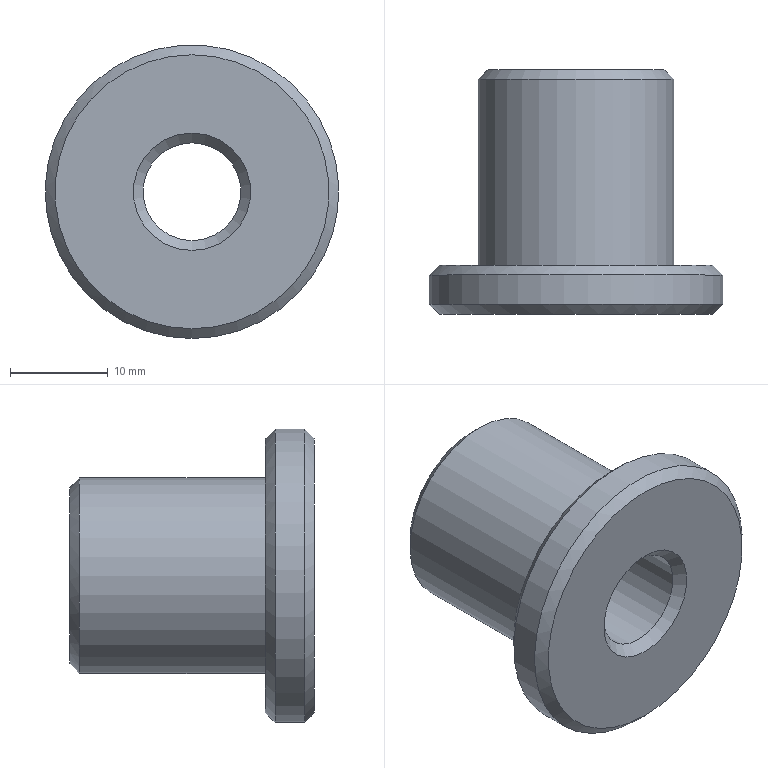Part | NX | features solid 2 | 1 solid | 10 faces | box 30 x 25 x 30 mm | volume 7715 mm3 | cone 4 | plane 3 | cylinder 3 | commonest cylinder face diameters 10 x1 20 x1 30 x1
STEP:
#1=CARTESIAN_POINT('',(0.000006093,336.216,159.366));
#2=VERTEX_POINT('',#1);
#3=CARTESIAN_POINT('',(0.000006093,336.216,173.366));
#4=DIRECTION('',(0.,-1.,0.));
#5=DIRECTION('',(0.,0.,-1.));
#6=AXIS2_PLACEMENT_3D('',#3,#4,#5);
#7=CIRCLE('',#6,14.);
#8=EDGE_CURVE('',#2,#2,#7,.F.);
#9=ORIENTED_EDGE('',*,*,#8,.T.);
#10=EDGE_LOOP('',(#9));
#11=FACE_BOUND('',#10,.T.);
#12=CARTESIAN_POINT('',(0.000006093,336.216,163.366));
#13=VERTEX_POINT('',#12);
#14=CARTESIAN_POINT('',(0.000006093,336.216,173.366));
#15=DIRECTION('',(0.,-1.,0.));
#16=DIRECTION('',(0.,0.,-1.));
#17=AXIS2_PLACEMENT_3D('',#14,#15,#16);
#18=CIRCLE('',#17,10.);
#19=EDGE_CURVE('',#13,#13,#18,.T.);
#20=ORIENTED_EDGE('',*,*,#19,.T.);
#21=EDGE_LOOP('',(#20));
#22=FACE_BOUND('',#21,.T.);
#23=CARTESIAN_POINT('',(-0.000000942,336.216,122.381));
#24=DIRECTION('',(0.,-1.,0.));
#25=DIRECTION('',(-1.,0.,0.));
#26=AXIS2_PLACEMENT_3D('',#23,#24,#25);
#27=PLANE('',#26);
#28=ADVANCED_FACE('',(#11,#22),#27,.F.);
#29=CARTESIAN_POINT('',(0.000006093,331.216,167.366));
#30=VERTEX_POINT('',#29);
#31=CARTESIAN_POINT('',(0.000006093,331.216,173.366));
#32=DIRECTION('',(0.,-1.,0.));
#33=DIRECTION('',(0.,0.,-1.));
#34=AXIS2_PLACEMENT_3D('',#31,#32,#33);
#35=CIRCLE('',#34,6.);
#36=EDGE_CURVE('',#30,#30,#35,.F.);
#37=ORIENTED_EDGE('',*,*,#36,.T.);
#38=EDGE_LOOP('',(#37));
#39=FACE_BOUND('',#38,.T.);
#40=CARTESIAN_POINT('',(0.000006093,331.216,159.366));
#41=VERTEX_POINT('',#40);
#42=CARTESIAN_POINT('',(0.000006093,331.216,173.366));
#43=DIRECTION('',(0.,-1.,0.));
#44=DIRECTION('',(0.,0.,-1.));
#45=AXIS2_PLACEMENT_3D('',#42,#43,#44);
#46=CIRCLE('',#45,14.);
#47=EDGE_CURVE('',#41,#41,#46,.T.);
#48=ORIENTED_EDGE('',*,*,#47,.T.);
#49=EDGE_LOOP('',(#48));
#50=FACE_BOUND('',#49,.T.);
#51=CARTESIAN_POINT('',(-0.000000942,331.216,122.381));
#52=DIRECTION('',(0.,-1.,0.));
#53=DIRECTION('',(-1.,0.,0.));
#54=AXIS2_PLACEMENT_3D('',#51,#52,#53);
#55=PLANE('',#54);
#56=ADVANCED_FACE('',(#39,#50),#55,.T.);
#57=CARTESIAN_POINT('',(0.000006093,335.216,158.366));
#58=VERTEX_POINT('',#57);
#59=CARTESIAN_POINT('',(0.000006093,335.216,173.366));
#60=DIRECTION('',(0.,-1.,0.));
#61=DIRECTION('',(0.,0.,-1.));
#62=AXIS2_PLACEMENT_3D('',#59,#60,#61);
#63=CIRCLE('',#62,15.);
#64=EDGE_CURVE('',#58,#58,#63,.T.);
#65=ORIENTED_EDGE('',*,*,#64,.T.);
#66=EDGE_LOOP('',(#65));
#67=FACE_BOUND('',#66,.T.);
#68=CARTESIAN_POINT('',(0.000006093,332.216,158.366));
#69=VERTEX_POINT('',#68);
#70=CARTESIAN_POINT('',(0.000006093,332.216,173.366));
#71=DIRECTION('',(0.,-1.,0.));
#72=DIRECTION('',(0.,0.,-1.));
#73=AXIS2_PLACEMENT_3D('',#70,#71,#72);
#74=CIRCLE('',#73,15.);
#75=EDGE_CURVE('',#69,#69,#74,.F.);
#76=ORIENTED_EDGE('',*,*,#75,.T.);
#77=EDGE_LOOP('',(#76));
#78=FACE_BOUND('',#77,.T.);
#79=CARTESIAN_POINT('',(0.000006093,361.216,173.366));
#80=DIRECTION('',(0.,-1.,0.));
#81=DIRECTION('',(1.,0.,0.));
#82=AXIS2_PLACEMENT_3D('',#79,#80,#81);
#83=CYLINDRICAL_SURFACE('',#82,15.);
#84=ADVANCED_FACE('',(#67,#78),#83,.T.);
#85=CARTESIAN_POINT('',(0.000006093,356.216,182.366));
#86=VERTEX_POINT('',#85);
#87=CARTESIAN_POINT('',(0.000006093,356.216,173.366));
#88=DIRECTION('',(0.,1.,0.));
#89=DIRECTION('',(0.,0.,1.));
#90=AXIS2_PLACEMENT_3D('',#87,#88,#89);
#91=CIRCLE('',#90,9.);
#92=EDGE_CURVE('',#86,#86,#91,.T.);
#93=ORIENTED_EDGE('',*,*,#92,.T.);
#94=EDGE_LOOP('',(#93));
#95=FACE_BOUND('',#94,.T.);
#96=CARTESIAN_POINT('',(0.000006093,356.216,178.366));
#97=VERTEX_POINT('',#96);
#98=CARTESIAN_POINT('',(0.000006093,356.216,173.366));
#99=DIRECTION('',(0.,1.,0.));
#100=DIRECTION('',(0.,0.,1.));
#101=AXIS2_PLACEMENT_3D('',#98,#99,#100);
#102=CIRCLE('',#101,5.);
#103=EDGE_CURVE('',#97,#97,#102,.T.);
#104=ORIENTED_EDGE('',*,*,#103,.F.);
#105=EDGE_LOOP('',(#104));
#106=FACE_BOUND('',#105,.T.);
#107=CARTESIAN_POINT('',(0.000006093,356.216,173.366));
#108=DIRECTION('',(0.,1.,0.));
#109=DIRECTION('',(0.,0.,1.));
#110=AXIS2_PLACEMENT_3D('',#107,#108,#109);
#111=PLANE('',#110);
#112=ADVANCED_FACE('',(#95,#106),#111,.T.);
#113=CARTESIAN_POINT('',(0.000006093,355.216,183.366));
#114=VERTEX_POINT('',#113);
#115=CARTESIAN_POINT('',(0.000006093,355.216,173.366));
#116=DIRECTION('',(0.,1.,0.));
#117=DIRECTION('',(0.,0.,1.));
#118=AXIS2_PLACEMENT_3D('',#115,#116,#117);
#119=CIRCLE('',#118,10.);
#120=EDGE_CURVE('',#114,#114,#119,.F.);
#121=ORIENTED_EDGE('',*,*,#120,.T.);
#122=EDGE_LOOP('',(#121));
#123=FACE_BOUND('',#122,.T.);
#124=ORIENTED_EDGE('',*,*,#19,.F.);
#125=EDGE_LOOP('',(#124));
#126=FACE_BOUND('',#125,.T.);
#127=CARTESIAN_POINT('',(0.000006093,361.216,173.366));
#128=DIRECTION('',(0.,-1.,0.));
#129=DIRECTION('',(1.,0.,0.));
#130=AXIS2_PLACEMENT_3D('',#127,#128,#129);
#131=CYLINDRICAL_SURFACE('',#130,10.);
#132=ADVANCED_FACE('',(#123,#126),#131,.T.);
#133=CARTESIAN_POINT('',(0.000006093,332.216,168.366));
#134=VERTEX_POINT('',#133);
#135=CARTESIAN_POINT('',(0.000006093,332.216,173.366));
#136=DIRECTION('',(0.,-1.,0.));
#137=DIRECTION('',(0.,0.,-1.));
#138=AXIS2_PLACEMENT_3D('',#135,#136,#137);
#139=CIRCLE('',#138,5.);
#140=EDGE_CURVE('',#134,#134,#139,.T.);
#141=ORIENTED_EDGE('',*,*,#140,.T.);
#142=EDGE_LOOP('',(#141));
#143=FACE_BOUND('',#142,.T.);
#144=ORIENTED_EDGE('',*,*,#103,.T.);
#145=EDGE_LOOP('',(#144));
#146=FACE_BOUND('',#145,.T.);
#147=CARTESIAN_POINT('',(0.000006093,412.332,173.366));
#148=DIRECTION('',(0.,1.,0.));
#149=DIRECTION('',(0.8321,0.,-0.5546));
#150=AXIS2_PLACEMENT_3D('',#147,#148,#149);
#151=CYLINDRICAL_SURFACE('',#150,5.);
#152=ADVANCED_FACE('',(#143,#146),#151,.F.);
#153=ORIENTED_EDGE('',*,*,#92,.F.);
#154=EDGE_LOOP('',(#153));
#155=FACE_BOUND('',#154,.T.);
#156=ORIENTED_EDGE('',*,*,#120,.F.);
#157=EDGE_LOOP('',(#156));
#158=FACE_BOUND('',#157,.T.);
#159=CARTESIAN_POINT('',(0.000006093,355.216,173.366));
#160=DIRECTION('',(0.,-1.,0.));
#161=DIRECTION('',(0.,0.,-1.));
#162=AXIS2_PLACEMENT_3D('',#159,#160,#161);
#163=CONICAL_SURFACE('',#162,10.,0.7854);
#164=ADVANCED_FACE('',(#155,#158),#163,.T.);
#165=ORIENTED_EDGE('',*,*,#64,.F.);
#166=EDGE_LOOP('',(#165));
#167=FACE_BOUND('',#166,.T.);
#168=ORIENTED_EDGE('',*,*,#8,.F.);
#169=EDGE_LOOP('',(#168));
#170=FACE_BOUND('',#169,.T.);
#171=CARTESIAN_POINT('',(0.000006093,336.216,173.366));
#172=DIRECTION('',(0.,-1.,0.));
#173=DIRECTION('',(0.,0.,-1.));
#174=AXIS2_PLACEMENT_3D('',#171,#172,#173);
#175=CONICAL_SURFACE('',#174,14.,0.7854);
#176=ADVANCED_FACE('',(#167,#170),#175,.T.);
#177=ORIENTED_EDGE('',*,*,#36,.F.);
#178=EDGE_LOOP('',(#177));
#179=FACE_BOUND('',#178,.T.);
#180=ORIENTED_EDGE('',*,*,#140,.F.);
#181=EDGE_LOOP('',(#180));
#182=FACE_BOUND('',#181,.T.);
#183=CARTESIAN_POINT('',(0.000006093,332.216,173.366));
#184=DIRECTION('',(0.,-1.,0.));
#185=DIRECTION('',(0.,0.,-1.));
#186=AXIS2_PLACEMENT_3D('',#183,#184,#185);
#187=CONICAL_SURFACE('',#186,5.,0.7854);
#188=ADVANCED_FACE('',(#179,#182),#187,.F.);
#189=ORIENTED_EDGE('',*,*,#47,.F.);
#190=EDGE_LOOP('',(#189));
#191=FACE_BOUND('',#190,.T.);
#192=ORIENTED_EDGE('',*,*,#75,.F.);
#193=EDGE_LOOP('',(#192));
#194=FACE_BOUND('',#193,.T.);
#195=CARTESIAN_POINT('',(0.000006093,332.216,173.366));
#196=DIRECTION('',(0.,1.,0.));
#197=DIRECTION('',(0.,0.,1.));
#198=AXIS2_PLACEMENT_3D('',#195,#196,#197);
#199=CONICAL_SURFACE('',#198,15.,0.7854);
#200=ADVANCED_FACE('',(#191,#194),#199,.T.);
#201=CLOSED_SHELL('',(#28,#56,#84,#112,#132,#152,#164,#176,#188,#200));
#202=MANIFOLD_SOLID_BREP('',#201);
#203=(LENGTH_UNIT()NAMED_UNIT(*)SI_UNIT(.MILLI.,.METRE.));
#204=UNCERTAINTY_MEASURE_WITH_UNIT(LENGTH_MEASURE(0.00001),#203,'','');
#205=(NAMED_UNIT(*)PLANE_ANGLE_UNIT()SI_UNIT($,.RADIAN.));
#206=(NAMED_UNIT(*)SI_UNIT($,.STERADIAN.)SOLID_ANGLE_UNIT());
#207=(GEOMETRIC_REPRESENTATION_CONTEXT(3)GLOBAL_UNCERTAINTY_ASSIGNED_CONTEXT((#204))GLOBAL_UNIT_ASSIGNED_CONTEXT((#203,#205,#206))REPRESENTATION_CONTEXT('',''));
#208=ADVANCED_BREP_SHAPE_REPRESENTATION('',(#202),#207);